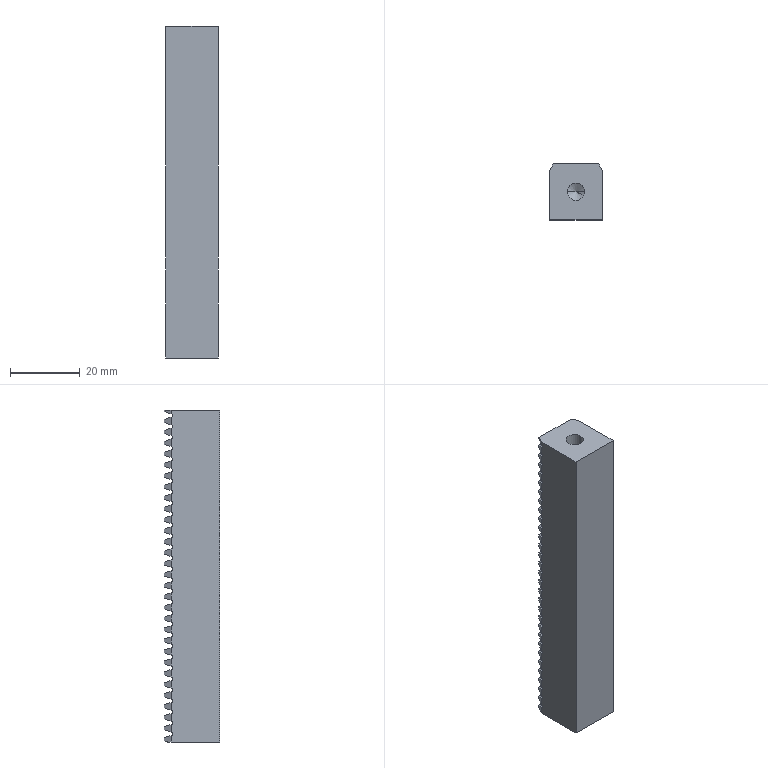Part | STEP file | 04-07 Rotary feed rack | 1 solid | 284 faces | box 15 x 16 x 95 mm | volume 20700 mm3 | plane 220 | cylinder 62 | cone 2 | commonest cylinder face diameters 1 x60 5 x2